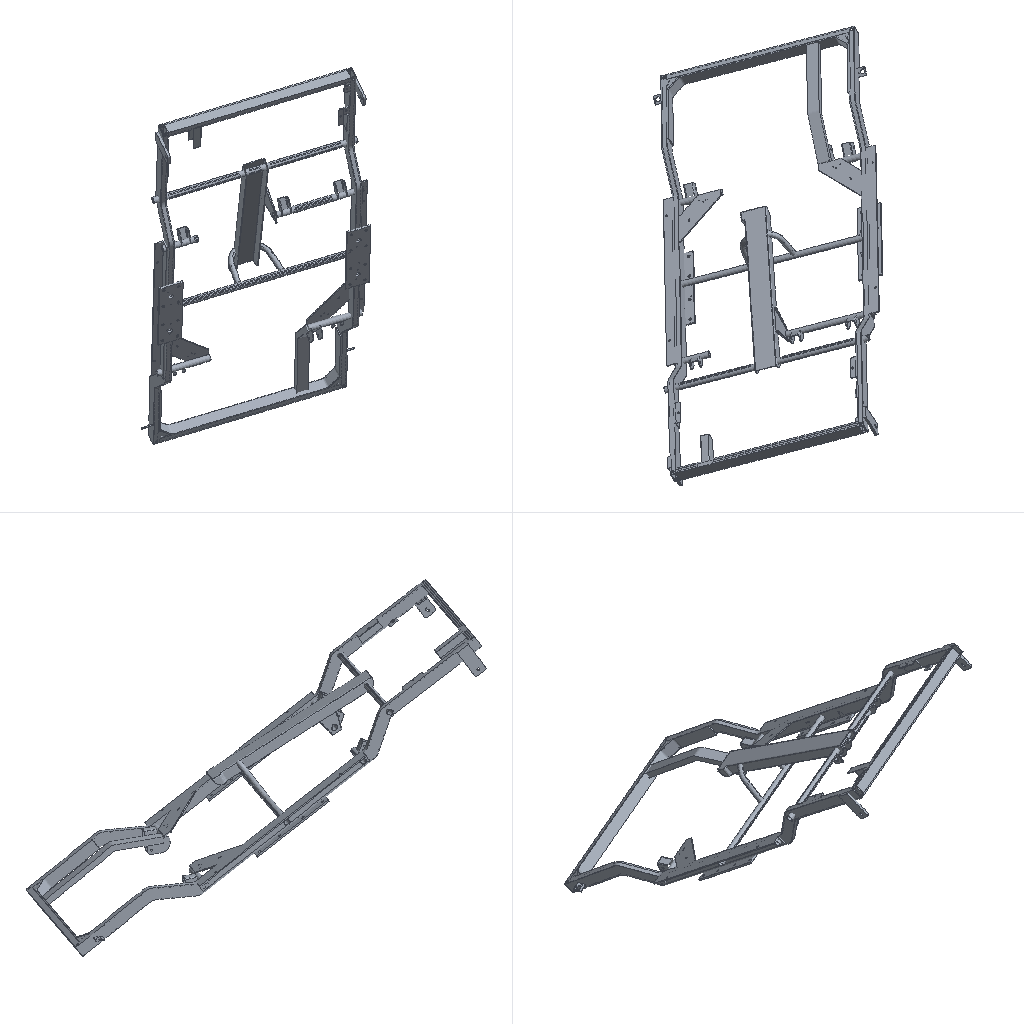Simulation study | ansys workbench
Set-up summary:
category,name,step,type,value,unit,region
solver,ansys_workbench
units,SI m-kg-s (Pa),,stated,"/units,MKS"
analysis,LS1,,static
load_step,LS1,LS1,static,nsubst=1; time=1
mesh,nodes,,,737056
mesh,elements,,,373772
element_type,SOLID187,,,242914
element_type,TARGE170,,,42796
element_type,CONTA174,,,42796
element_type,SOLID186,,,42166
element_type,SURF154,,,3100
material,Structural Steel,,E,2e+11,Pa
material,Structural Steel,,nu,0.3
material,Structural Steel,,density,7850,kg m^-3
material,Structural Steel,,conductivity,60.5,W m^-1 C^-1
material,Structural Steel,,specific_heat,434,J kg^-1 C^-1
material,Structural Steel,,cte,1.2e-05,C^-1
material,Structural Steel,,permeability,10000
material,Structural Steel,,resistivity,1.7e-07,kg m^3 A^-2 s^-3
load,Define Force Using Surface Effect Elements,LS1,surface-effect pres face 1,-51822.3,,SURF154 #195
load,Define Force Using Surface Effect Elements,LS1,surface-effect pres face 2,2.04463e+06,,SURF154 #195
load,Define Force Using Surface Effect Elements,LS1,surface-effect pres face 3,-1.57917e+06,,SURF154 #195
load,Define Force Using Surface Effect Elements,LS1,surface-effect pres face 1,-16714.4,,SURF154 #196
load,Define Force Using Surface Effect Elements,LS1,surface-effect pres face 2,1.2043e+06,,SURF154 #196
load,Define Force Using Surface Effect Elements,LS1,surface-effect pres face 3,-976255,,SURF154 #196
bc,Fixed Supports,model,fixed,[dofs=ALL],,_FIXEDSU
contact,Contact Region,,bonded (always),element=CONTA174
contact,Contact Region 2,,bonded (always),element=CONTA174
contact,Contact Region 3,,bonded (always),element=CONTA174
contact,Contact Region 4,,bonded (always),element=CONTA174
contact,Contact Region 5,,bonded (always),element=CONTA174
contact,Contact Region 6,,bonded (always),element=CONTA174
contact,Contact Region 7,,bonded (always),element=CONTA174
contact,Contact Region 8,,bonded (always),element=CONTA174
contact,Contact Region 9,,bonded (always),element=CONTA174
contact,Contact Region 10,,bonded (always),element=CONTA174
contact,Contact Region 11,,bonded (always),element=CONTA174
contact,Contact Region 12,,bonded (always),element=CONTA174
contact,Contact Region 13,,bonded (always),element=CONTA174
contact,Contact Region 14,,bonded (always),element=CONTA174
contact,Contact Region 15,,bonded (always),element=CONTA174
contact,Contact Region 16,,bonded (always),element=CONTA174
contact,Contact Region 17,,bonded (always),element=CONTA174
contact,Contact Region 18,,bonded (always),element=CONTA174
contact,Contact Region 19,,bonded (always),element=CONTA174
contact,Contact Region 20,,bonded (always),element=CONTA174
contact,Contact Region 21,,bonded (always),element=CONTA174
contact,Contact Region 22,,bonded (always),element=CONTA174
contact,Contact Region 23,,bonded (always),element=CONTA174
contact,Contact Region 24,,bonded (always),element=CONTA174
contact,Contact Region 25,,bonded (always),element=CONTA174
contact,Contact Region 26,,bonded (always),element=CONTA174
contact,Contact Region 27,,bonded (always),element=CONTA174
contact,Contact Region 28,,bonded (always),element=CONTA174
contact,Contact Region 29,,bonded (always),element=CONTA174
contact,Contact Region 30,,bonded (always),element=CONTA174
contact,Contact Region 31,,bonded (always),element=CONTA174
contact,Contact Region 32,,bonded (always),element=CONTA174
contact,Contact Region 33,,bonded (always),element=CONTA174
contact,Contact Region 34,,bonded (always),element=CONTA174
contact,Contact Region 35,,bonded (always),element=CONTA174
contact,Contact Region 36,,bonded (always),element=CONTA174
contact,Contact Region 37,,bonded (always),element=CONTA174
contact,Contact Region 38,,bonded (always),element=CONTA174
contact,Contact Region 39,,bonded (always),element=CONTA174
contact,Contact Region 40,,bonded (always),element=CONTA174
contact,Contact Region 41,,bonded (always),element=CONTA174
contact,Contact Region 42,,bonded (always),element=CONTA174
contact,Contact Region 43,,bonded (always),element=CONTA174
contact,Contact Region 44,,bonded (always),element=CONTA174
contact,Contact Region 45,,bonded (always),element=CONTA174
contact,Contact Region 46,,bonded (always),element=CONTA174
contact,Contact Region 47,,bonded (always),element=CONTA174
contact,Contact Region 48,,bonded (always),element=CONTA174
contact,Contact Region 49,,bonded (always),element=CONTA174
contact,Contact Region 50,,bonded (always),element=CONTA174
contact,Contact Region 51,,bonded (always),element=CONTA174
contact,Contact Region 52,,bonded (always),element=CONTA174
contact,Contact Region 53,,bonded (always),element=CONTA174
contact,Contact Region 54,,bonded (always),element=CONTA174
contact,Contact Region 55,,bonded (always),element=CONTA174
contact,Contact Region 56,,bonded (always),element=CONTA174
contact,Contact Region 57,,bonded (always),element=CONTA174
contact,Contact Region 58,,bonded (always),element=CONTA174
contact,Contact Region 59,,bonded (always),element=CONTA174
contact,Contact Region 60,,bonded (always),element=CONTA174
contact,Contact Region 61,,bonded (always),element=CONTA174
contact,Contact Region 62,,bonded (always),element=CONTA174
contact,Contact Region 63,,bonded (always),element=CONTA174
contact,Contact Region 64,,bonded (always),element=CONTA174
contact,Contact Region 65,,bonded (always),element=CONTA174
contact,Contact Region 66,,bonded (always),element=CONTA174
contact,Contact Region 67,,bonded (always),element=CONTA174
contact,Contact Region 68,,bonded (always),element=CONTA174
contact,Contact Region 69,,bonded (always),element=CONTA174
contact,Contact Region 70,,bonded (always),element=CONTA174
contact,Contact Region 71,,bonded (always),element=CONTA174
contact,Contact Region 72,,bonded (always),element=CONTA174
contact,Contact Region 73,,bonded (always),element=CONTA174
contact,Contact Region 74,,bonded (always),element=CONTA174
contact,Contact Region 75,,bonded (always),element=CONTA174
named_set,_FIXEDSU,,node,9496
Ansys APDL input file, long lists of numbers shortened:
/batch
/config,noeldb,1     ! force off writing results to database
*get,_wallstrt,active,,time,wall
! ANSYS input file written by Workbench version 2024 R2
! File used for geometry attach:
/title,wbnew--____ (A5)
! ****** Begin Custom Load Command Snippet ******
/COM, ACT Extensions:
/COM,     LSDYNA, 2024.2
/COM,/COM,     ANSYSMotion, 2024.2
/COM,
! ****** End   Custom Load Command Snippet ******
*DIM,_wb_ProjectScratch_dir,string,248
_wb_ProjectScratch_dir(1) = ''
*DIM,_wb_SolverFiles_dir,string,248
_wb_SolverFiles_dir(1) = ''
*DIM,_wb_userfiles_dir,string,248
_wb_userfiles_dir(1) = ''
/com,--- Data in consistent MKS units. See Solving Units in the help system for more information.
/units,MKS
/nopr
/wb,file,start              !  signify a WB generated input file
/prep7
! Turn off shape checking because checks already performed inside WB mesher.
! See help system for more information.
SHPP,OFF,,NOWARN
/nolist
etcon,set             ! allow ANSYS to choose best KEYOP's for 180x elements, resets any applicable keyopt to MAPDL defaults
/com,*********** Nodes for the whole assembly ***********
nblock,3,,810761
(1i9,3e20.9e3)
   685375    -3.735245650E-01     6.288331249E-01    -6.786277806E-01
! (737055 more lines like these left out)
-1
/wb,elem,start            !  set before creation of elements
/com,*********** Elements for Body 1 'car chassis-FreeParts|Shell1' ***********
et,1,186
keyo,1,2,1          ! set full integration on SOLID186
eblock,19,solid,,4650
(19i9)
        1        1        1        1        0        0        0        0       20        0        1     4393     4547     8424     8578     5014     5013     9044     9045
! (9299 more lines like these left out)
-1
/com,*********** Elements for Body 2 'car chassis-FreeParts|Body-Move/Copy6' ***********
et,2,187
eblock,19,solid,,1516
(19i9)
        2        2        2        2        0        0        0        0       10        0     4651    31992    32336    32302    32281    33664    34931    33663    33662
! (3031 more lines like these left out)
-1
/com,*********** Elements for Body 3 'car chassis-FreeParts|Extrude-Thin2' ***********
et,3,186
keyo,3,2,1          ! set full integration on SOLID186
eblock,19,solid,,3150
(19i9)
        3        3        3        3        0        0        0        0       20        0     6167    36484    36485    39633    39634    37878    37877    40677    40678
! (6299 more lines like these left out)
-1
/com,*********** Elements for Body 4 'car chassis-FreeParts|Cut-Extrude23' ***********
et,4,186
keyo,4,2,1          ! set full integration on SOLID186
eblock,19,solid,,106
(19i9)
        4        4        4        4        0        0        0        0       20        0     9317    55081    55102    55101    55100    55140    55119    55120    55121
! (211 more lines like these left out)
-1
/com,*********** Elements for Body 5 'car chassis-FreeParts|Mirror1[5]' ***********
et,5,186
keyo,5,2,1          ! set full integration on SOLID186
eblock,19,solid,,1800
(19i9)
        5        5        5        5        0        0        0        0       20        0     9423    55832    55833    55835    55840    57226    57225    57223    57218
! (3599 more lines like these left out)
-1
/com,*********** Elements for Body 6 'car chassis-FreeParts|Sweep-Thin1' ***********
et,6,187
eblock,19,solid,,3008
(19i9)
        6        6        6        6        0        0        0        0       10        0    11223    64352    64602    64609    64752    65503    67232    65504    65506
! (6015 more lines like these left out)
-1
/com,*********** Elements for Body 7 'car chassis-FreeParts|Mirror1[1]' ***********
et,7,187
eblock,19,solid,,1712
(19i9)
        7        7        7        7        0        0        0        0       10        0    14231    70826    71059    71007    71076    73222    73989    73221    73223
! (3423 more lines like these left out)
-1
/com,*********** Elements for Body 8 'car chassis-FreeParts|Boss-Extrude21' ***********
et,8,186
keyo,8,2,1          ! set full integration on SOLID186
eblock,19,solid,,24
(19i9)
        8        8        8        8        0        0        0        0       20        0    15943    74065    74073    74093    74097    74069    74072    74092    74094
! (47 more lines like these left out)
-1
/com,*********** Elements for Body 9 'car chassis-FreeParts|Body-Move/Copy5' ***********
et,9,187
eblock,19,solid,,1521
(19i9)
        9        9        9        9        0        0        0        0       10        0    15967    74233    74605    74549    74532    74851    76559    74848    74847
! (3041 more lines like these left out)
-1
/com,*********** Elements for Body 10 'car chassis-FreeParts|Fillet12' ***********
et,10,187
eblock,19,solid,,421
(19i9)
       10       10       10       10        0        0        0        0       10        0    17488    77605    77645    77616    77672    78178    78224    78174    78179
! (841 more lines like these left out)
-1
/com,*********** Elements for Body 11 'car chassis-FreeParts|Cut-Extrude16' ***********
et,11,187
eblock,19,solid,,1518
(19i9)
       11       11       11       11        0        0        0        0       10        0    17909    78484    78485    78647    78620    79603    79617    79608    79605
! (3035 more lines like these left out)
-1
/com,*********** Elements for Body 12 'car chassis-FreeParts|Cut-Extrude2' ***********
et,12,186
keyo,12,2,1         ! set full integration on SOLID186
eblock,19,solid,,124
(19i9)
       12       12       12       12        0        0        0        0       20        0    19427    81667    81668    81704    81674    81742    81741    81705    81735
! (247 more lines like these left out)
-1
/com,*********** Elements for Body 13 'car chassis-FreeParts|Extrude-Thin4' ***********
et,13,186
keyo,13,2,1         ! set full integration on SOLID186
eblock,19,solid,,3132
(19i9)
       13       13       13       13        0        0        0        0       20        0    19551    83574    87054    87053    83575    83581    87059    87060    83582
! (6263 more lines like these left out)
-1
/com,*********** Elements for Body 14 'car chassis-FreeParts|Mirror1[4]' ***********
et,14,186
keyo,14,2,1         ! set full integration on SOLID186
eblock,19,solid,,773
(19i9)
       14       14       14       14        0        0        0        0       20        0    22683   102990   103020   103132   103133   103277   103247   103135   103134
! (1545 more lines like these left out)
-1
/com,*********** Elements for Body 15 'car chassis-FreeParts|Mirror3' ***********
et,15,187
eblock,19,solid,,3010
(19i9)
       15       15       15       15        0        0        0        0       10        0    23456   108364   108576   108388   108377   110721   110967   110712   110711
! (6019 more lines like these left out)
-1
/com,*********** Elements for Body 16 'car chassis-FreeParts|Mirror1[7]' ***********
et,16,186
keyo,16,2,1         ! set full integration on SOLID186
eblock,19,solid,,80
(19i9)
       16       16       16       16        0        0        0        0       20        0    26466   114286   114335   114334   114398   114302   114327   114328   114396
! (159 more lines like these left out)
-1
/com,*********** Elements for Body 17 'car chassis-FreeParts|Boss-Extrude16' ***********
et,17,186
keyo,17,2,1         ! set full integration on SOLID186
eblock,19,solid,,624
(19i9)
       17       17       17       17        0        0        0        0       20        0    26546   115451   115485   115511   115637   115460   115486   115512   115638
! (1247 more lines like these left out)
-1
/com,*********** Elements for Body 18 'car chassis-FreeParts|Cut-Extrude5' ***********
et,18,187
eblock,19,solid,,1527
(19i9)
       18       18       18       18        0        0        0        0       10        0    27170   119503   119538   119968   119776   120806   120976   120809   120808
! (3053 more lines like these left out)
-1
/com,*********** Elements for Body 19 'car chassis-FreeParts|Shell3' ***********
et,19,187
eblock,19,solid,,71914
(19i9)
       19       19       19       19        0        0        0        0       10        0    28697   122954   146330   122979   122965   148277   148438   148274   148273
! (143827 more lines like these left out)
-1
/com,*********** Elements for Body 20 'car chassis-FreeParts|Boss-Extrude4' ***********
et,20,186
keyo,20,2,1         ! set full integration on SOLID186
eblock,19,solid,,5600
(19i9)
       20       20       20       20        0        0        0        0       20        0   100611   264773   271074   271062   271012   269212   271110   271061   271021
! (11199 more lines like these left out)
-1
/com,*********** Elements for Body 21 'car chassis-FreeParts|Cut-Extrude19' ***********
et,21,187
eblock,19,solid,,32876
(19i9)
       21       21       21       21        0        0        0        0       10        0   106211   292671   293638   292975   303848   304198   306550   304196   304201
! (65751 more lines like these left out)
-1
/com,*********** Elements for Body 22 'car chassis-FreeParts|Extrude-Thin12' ***********
et,22,186
keyo,22,2,1         ! set full integration on SOLID186
eblock,19,solid,,5380
(19i9)
       22       22       22       22        0        0        0        0       20        0   139087   359310   365520   365518   365453   361989   365529   365519   365509
! (10759 more lines like these left out)
-1
/com,*********** Elements for Body 23 'car chassis-FreeParts|Extrude-Thin9' ***********
et,23,186
keyo,23,2,1         ! set full integration on SOLID186
eblock,19,solid,,540
(19i9)
       23       23       23       23        0        0        0        0       20        0   144467   391412   391413   391951   391952   391646   391645   392125   392126
! (1079 more lines like these left out)
-1
/com,*********** Elements for Body 24 'car chassis-FreeParts|Cut-Extrude13[1]' ***********
et,24,187
eblock,19,solid,,20919
(19i9)
       24       24       24       24        0        0        0        0       10        0   145007   395852   401161   396791   397764   409238   415890   409232   409236
! (41837 more lines like these left out)
-1
/com,*********** Elements for Body 25 'car chassis-FreeParts|Boss-Extrude10' ***********
et,25,186
keyo,25,2,1         ! set full integration on SOLID186
eblock,19,solid,,1665
(19i9)
       25       25       25       25        0        0        0        0       20        0   165926   434165   434166   434172   434190   435469   435468   435462   435444
! (3329 more lines like these left out)
-1
/com,*********** Elements for Body 26 'car chassis-FreeParts|Extrude-Thin3' ***********
et,26,186
keyo,26,2,1         ! set full integration on SOLID186
eblock,19,solid,,1368
(19i9)
       26       26       26       26        0        0        0        0       20        0   167591   442738   444256   444255   442739   442745   444263   444264   442746
! (2735 more lines like these left out)
-1
/com,*********** Elements for Body 27 'car chassis-FreeParts|Cut-Extrude21[2]' ***********
et,27,186
keyo,27,2,1         ! set full integration on SOLID186
eblock,19,solid,,3000
(19i9)
       27       27       27       27        0        0        0        0       20        0   168959   451283   452270   452269   452283   453428   452441   452442   452428
! (5999 more lines like these left out)
-1
/com,*********** Elements for Body 28 'car chassis-FreeParts|Mirror4' ***********
et,28,187
eblock,19,solid,,1614
(19i9)
       28       28       28       28        0        0        0        0       10        0   171959   468557   469153   468559   468897   469274   469284   469268   469273
! (3227 more lines like these left out)
-1
! (1 more sections like these left out)
/com,*********** Elements for Body 30 'car chassis-FreeParts|Boss-Extrude15' ***********
et,30,186
keyo,30,2,1         ! set full integration on SOLID186
eblock,19,solid,,590
(19i9)
       30       30       30       30        0        0        0        0       20        0   173665   472683   472716   472802   472803   473148   473115   473029   473028
! (1179 more lines like these left out)
-1
/com,*********** Elements for Body 31 'car chassis-FreeParts|Body-Move/Copy7' ***********
et,31,187
eblock,19,solid,,409
(19i9)
       31       31       31       31        0        0        0        0       10        0   174255   476289   476385   476293   476360   476691   476714   476688   476690
! (817 more lines like these left out)
-1
! (3 more sections like these left out)
/com,*********** Elements for Body 35 'car chassis-FreeParts|Mirror1[8]' ***********
et,35,186
keyo,35,2,1         ! set full integration on SOLID186
eblock,19,solid,,124
(19i9)
       35       35       35       35        0        0        0        0       20        0   178094   489044   489269   489053   489047   489119   489282   489110   489116
! (247 more lines like these left out)
-1
/com,*********** Elements for Body 36 'car chassis-FreeParts|Shell4' ***********
et,36,187
eblock,19,solid,,71996
(19i9)
       36       36       36       36        0        0        0        0       10        0   178218   490599   511935   512117   513547   518014   629890   518015   518016
! (143991 more lines like these left out)
-1
! (1 more sections like these left out)
/com,*********** Elements for Body 38 'car chassis-FreeParts|Shell2' ***********
et,38,186
keyo,38,2,1         ! set full integration on SOLID186
eblock,19,solid,,4650
(19i9)
       38       38       38       38        0        0        0        0       20        0   250294   634481   634635   639440   639594   635098   635099   639596   639595
! (9299 more lines like these left out)
-1
! (4 more sections like these left out)
/com,*********** Elements for Body 43 'car chassis-FreeParts|Mirror2' ***********
et,43,186
keyo,43,2,1         ! set full integration on SOLID186
eblock,19,solid,,598
(19i9)
       43       43       43       43        0        0        0        0       20        0   263584   694153   694256   694320   694254   694666   694563   694499   694565
! (1195 more lines like these left out)
-1
/com,*********** Elements for Body 44 'car chassis-FreeParts|Cut-Extrude13[3]' ***********
et,44,187
eblock,19,solid,,20899
(19i9)
       44       44       44       44        0        0        0        0       10        0   264182   699092   704235   699644   704188   713468   717616   713461   713467
! (41797 more lines like these left out)
-1
/wb,elem,end               !  done creating elements
/com,*********** Send User Defined Coordinate System(s) ***********
csys,0
toffst,273.15,      ! Temperature offset from absolute zero
/com,*********** Set Reference Temperature ***********
tref,22.
/wb,mat,start              !  starting to send materials
/com,*********** Send Materials ***********
Temperature = 'TEMP' ! Temperature
MP,DENS,1,7850,	! kg m^-3
MP,ALPX,1,1.2e-05,	! C^-1
MP,C,1,434,	! J kg^-1 C^-1
MP,KXX,1,60.5,	! W m^-1 C^-1
MP,RSVX,1,1.7e-07,	! kg m^3 A^-2 s^-3
MP,EX,1,200000000000,	! Pa
MP,NUXY,1,0.3,
MP,MURX,1,10000,
Temperature = 'TEMP' ! Temperature
MP,DENS,2,7850,	! kg m^-3
MP,ALPX,2,1.2e-05,	! C^-1
MP,C,2,434,	! J kg^-1 C^-1
MP,KXX,2,60.5,	! W m^-1 C^-1
MP,RSVX,2,1.7e-07,	! kg m^3 A^-2 s^-3
MP,EX,2,200000000000,	! Pa
MP,NUXY,2,0.3,
MP,MURX,2,10000,
Temperature = 'TEMP' ! Temperature
MP,DENS,3,7850,	! kg m^-3
MP,ALPX,3,1.2e-05,	! C^-1
MP,C,3,434,	! J kg^-1 C^-1
MP,KXX,3,60.5,	! W m^-1 C^-1
MP,RSVX,3,1.7e-07,	! kg m^3 A^-2 s^-3
MP,EX,3,200000000000,	! Pa
MP,NUXY,3,0.3,
MP,MURX,3,10000,
Temperature = 'TEMP' ! Temperature
MP,DENS,4,7850,	! kg m^-3
MP,ALPX,4,1.2e-05,	! C^-1
MP,C,4,434,	! J kg^-1 C^-1
MP,KXX,4,60.5,	! W m^-1 C^-1
MP,RSVX,4,1.7e-07,	! kg m^3 A^-2 s^-3
MP,EX,4,200000000000,	! Pa
MP,NUXY,4,0.3,
MP,MURX,4,10000,
Temperature = 'TEMP' ! Temperature
MP,DENS,5,7850,	! kg m^-3
MP,ALPX,5,1.2e-05,	! C^-1
MP,C,5,434,	! J kg^-1 C^-1
MP,KXX,5,60.5,	! W m^-1 C^-1
MP,RSVX,5,1.7e-07,	! kg m^3 A^-2 s^-3
MP,EX,5,200000000000,	! Pa
MP,NUXY,5,0.3,
MP,MURX,5,10000,
Temperature = 'TEMP' ! Temperature
MP,DENS,6,7850,	! kg m^-3
MP,ALPX,6,1.2e-05,	! C^-1
MP,C,6,434,	! J kg^-1 C^-1
MP,KXX,6,60.5,	! W m^-1 C^-1
MP,RSVX,6,1.7e-07,	! kg m^3 A^-2 s^-3
MP,EX,6,200000000000,	! Pa
MP,NUXY,6,0.3,
MP,MURX,6,10000,
Temperature = 'TEMP' ! Temperature
MP,DENS,7,7850,	! kg m^-3
MP,ALPX,7,1.2e-05,	! C^-1
MP,C,7,434,	! J kg^-1 C^-1
MP,KXX,7,60.5,	! W m^-1 C^-1
MP,RSVX,7,1.7e-07,	! kg m^3 A^-2 s^-3
MP,EX,7,200000000000,	! Pa
MP,NUXY,7,0.3,
MP,MURX,7,10000,
Temperature = 'TEMP' ! Temperature
MP,DENS,8,7850,	! kg m^-3
MP,ALPX,8,1.2e-05,	! C^-1
MP,C,8,434,	! J kg^-1 C^-1
MP,KXX,8,60.5,	! W m^-1 C^-1
MP,RSVX,8,1.7e-07,	! kg m^3 A^-2 s^-3
MP,EX,8,200000000000,	! Pa
MP,NUXY,8,0.3,
MP,MURX,8,10000,
Temperature = 'TEMP' ! Temperature
MP,DENS,9,7850,	! kg m^-3
MP,ALPX,9,1.2e-05,	! C^-1
MP,C,9,434,	! J kg^-1 C^-1
MP,KXX,9,60.5,	! W m^-1 C^-1
MP,RSVX,9,1.7e-07,	! kg m^3 A^-2 s^-3
MP,EX,9,200000000000,	! Pa
! (317 more lines like these left out)
/wb,mat,end                !  done sending materials
!************************* Model Summary ********************
!car chassis-FreeParts|Shell1,	ç»æé¢,	matid,	1
!car chassis-FreeParts|Body-Move/Copy6,	ç»æé¢,	matid,	2
!car chassis-FreeParts|Extrude-Thin2,	ç»æé¢,	matid,	3
! (43 more lines like these left out)
*get,_xmin,node,,mnloc,x
*get,_ymin,node,,mnloc,y
*get,_zmin,node,,mnloc,z
*get,_xmax,node,,mxloc,x
*get,_ymax,node,,mxloc,y
*get,_zmax,node,,mxloc,z
_ASMDIAG=(_xmax-_xmin)*(_xmax-_xmin)+(_ymax-_ymin)*(_ymax-_ymin)+(_zmax-_zmin)*(_zmax-_zmin)
_ASMDIAG=SQRT(_ASMDIAG)
/wb,contact,start          !  starting to send contact
/com,*********** Create Contact "½Ó´¥ÇøÓò" ***********
/com,            Real Constant Set For Above Contact Is 46 & 45
*set,tid,46
*set,cid,45
r,tid
r,cid
et,tid,170
et,cid,174
eblock,10,,,81
(15i9)
   498067       46       46       46        0     4071     4072     3918     3917    20898    20440    20436    20437
! (80 more lines like these left out)
-1
eblock,10,,,81
(15i9)
   498148       45       45       45        0     4071     4072     3918     3917    20898    20440    20436    20437
! (80 more lines like these left out)
-1
eblock,10,,,22
(15i9)
   498229       45       46       45        0    81843    81833    81855    81856    82384    82385    82422    82407
! (21 more lines like these left out)
-1
eblock,10,,,22
(15i9)
   498251       46       45       46        0    81843    81833    81855    81856    82384    82385    82422    82407
! (21 more lines like these left out)
-1
keyo,cid,8,2               ! auto create asymmetric contact (from Program Controlled setting)
keyo,cid,10,0              ! adjust contact stiffness each NR iteration (from Program Controlled setting)
keyo,cid,12,5              ! bonded always
keyo,cid,18,1              ! small sliding turned on by application
keyo,cid,2,2               ! MPC for bonded contacts (from Program Controlled setting)
keyo,tid,5,0               ! Automatic constraint type detection
keyo,cid,4,2               ! on nodal point - normal to target surface (from Program Controlled setting)
keyo,cid,9,1               ! ignore initial gaps/penetration
keyo,cid,7,0               ! No Prediction
rmod,tid,3,10.      ! FKN
rmod,tid,5,0.       ! ICONT
rmod,tid,6,0.       ! PINB
rmod,tid,10,0.      ! CNOF
rmod,tid,12,0.      ! FKT
rmod,tid,36,155     ! WB DSID
rmod,cid,3,10.      ! FKN
rmod,cid,5,0.       ! ICONT
rmod,cid,6,0.       ! PINB
rmod,cid,10,0.      ! CNOF
rmod,cid,12,0.      ! FKT
rmod,cid,36,155     ! WB DSID
/com,*********** Create Contact "½Ó´¥ÇøÓò 2" ***********
/com,            Real Constant Set For Above Contact Is 48 & 47
*set,tid,48
*set,cid,47
r,tid
r,cid
et,tid,170
et,cid,174
eblock,10,,,78
(15i9)
   498273       48       48       48        0       27     3624     1919       45     9133    14764     9170     9132
! (77 more lines like these left out)
-1
eblock,10,,,78
(15i9)
   498351       47       47       47        0       27     3624     1919       45     9133    14764     9170     9132
! (77 more lines like these left out)
-1
eblock,10,,,80
(15i9)
   498429       47       48       47        0   114344   114351   114260   114261   114675   114418   114416   114421
! (79 more lines like these left out)
-1
eblock,10,,,80
(15i9)
   498509       48       47       48        0   114344   114351   114260   114261   114675   114418   114416   114421
! (79 more lines like these left out)
-1
keyo,cid,8,2               ! auto create asymmetric contact (from Program Controlled setting)
keyo,cid,10,0              ! adjust contact stiffness each NR iteration (from Program Controlled setting)
keyo,cid,12,5              ! bonded always
keyo,cid,18,1              ! small sliding turned on by application
keyo,cid,2,2               ! MPC for bonded contacts (from Program Controlled setting)
keyo,tid,5,0               ! Automatic constraint type detection
keyo,cid,4,2               ! on nodal point - normal to target surface (from Program Controlled setting)
keyo,cid,9,1               ! ignore initial gaps/penetration
keyo,cid,7,0               ! No Prediction
rmod,tid,3,10.      ! FKN
rmod,tid,5,0.       ! ICONT
rmod,tid,6,0.       ! PINB
rmod,tid,10,0.      ! CNOF
rmod,tid,12,0.      ! FKT
rmod,tid,36,158     ! WB DSID
rmod,cid,3,10.      ! FKN
rmod,cid,5,0.       ! ICONT
rmod,cid,6,0.       ! PINB
rmod,cid,10,0.      ! CNOF
rmod,cid,12,0.      ! FKT
rmod,cid,36,158     ! WB DSID
/com,*********** Create Contact "½Ó´¥ÇøÓò 3" ***********
/com,            Real Constant Set For Above Contact Is 50 & 49
*set,tid,50
*set,cid,49
r,tid
r,cid
et,tid,170
et,cid,174
eblock,10,,,30
(15i9)
   498589       50       50       50        0     9043     9044     5013     5013    31762    23723     5013    23722
! (29 more lines like these left out)
-1
eblock,10,,,30
(15i9)
   498619       49       49       49        0     9043     9044     5013     5013    31762    23723     5013    23722
! (29 more lines like these left out)
-1
eblock,10,,,205
(15i9)
   498649       49       50       49        0   133272   134310   133704   133704   223948   225982   133704   223947
! (204 more lines like these left out)
-1
eblock,10,,,205
(15i9)
   498854       50       49       50        0   133272   134310   133704   133704   223948   225982   133704   223947
! (204 more lines like these left out)
-1
keyo,cid,8,2               ! auto create asymmetric contact (from Program Controlled setting)
keyo,cid,10,0              ! adjust contact stiffness each NR iteration (from Program Controlled setting)
keyo,cid,12,5              ! bonded always
keyo,cid,18,1              ! small sliding turned on by application
keyo,cid,2,2               ! MPC for bonded contacts (from Program Controlled setting)
keyo,tid,5,0               ! Automatic constraint type detection
keyo,cid,4,2               ! on nodal point - normal to target surface (from Program Controlled setting)
keyo,cid,9,1               ! ignore initial gaps/penetration
keyo,cid,7,0               ! No Prediction
rmod,tid,3,10.      ! FKN
rmod,tid,5,0.       ! ICONT
rmod,tid,6,0.       ! PINB
rmod,tid,10,0.      ! CNOF
rmod,tid,12,0.      ! FKT
rmod,tid,36,161     ! WB DSID
rmod,cid,3,10.      ! FKN
rmod,cid,5,0.       ! ICONT
rmod,cid,6,0.       ! PINB
rmod,cid,10,0.      ! CNOF
rmod,cid,12,0.      ! FKT
rmod,cid,36,161     ! WB DSID
/com,*********** Create Contact "½Ó´¥ÇøÓò 4" ***********
/com,            Real Constant Set For Above Contact Is 52 & 51
*set,tid,52
*set,cid,51
r,tid
r,cid
et,tid,170
et,cid,174
eblock,10,,,176
(15i9)
   499059       52       52       52        0     4353     4354     4200     4199    21744    21286    21282    21283
! (175 more lines like these left out)
-1
eblock,10,,,176
(15i9)
   499235       51       51       51        0     4353     4354     4200     4199    21744    21286    21282    21283
! (175 more lines like these left out)
-1
eblock,10,,,50
(15i9)
   499411       51       52       51        0   269889   269891   269950   269890   288170   288174   288171   288169
! (49 more lines like these left out)
-1
eblock,10,,,50
(15i9)
   499461       52       51       52        0   269889   269891   269950   269890   288170   288174   288171   288169
! (49 more lines like these left out)
-1
keyo,cid,8,2               ! auto create asymmetric contact (from Program Controlled setting)
keyo,cid,10,0              ! adjust contact stiffness each NR iteration (from Program Controlled setting)
keyo,cid,12,5              ! bonded always
keyo,cid,18,1              ! small sliding turned on by application
keyo,cid,2,2               ! MPC for bonded contacts (from Program Controlled setting)
keyo,tid,5,0               ! Automatic constraint type detection
keyo,cid,4,2               ! on nodal point - normal to target surface (from Program Controlled setting)
keyo,cid,9,1               ! ignore initial gaps/penetration
keyo,cid,7,0               ! No Prediction
rmod,tid,3,10.      ! FKN
rmod,tid,5,0.       ! ICONT
rmod,tid,6,0.       ! PINB
rmod,tid,10,0.      ! CNOF
rmod,tid,12,0.      ! FKT
rmod,tid,36,164     ! WB DSID
rmod,cid,3,10.      ! FKN
rmod,cid,5,0.       ! ICONT
rmod,cid,6,0.       ! PINB
rmod,cid,10,0.      ! CNOF
rmod,cid,12,0.      ! FKT
rmod,cid,36,164     ! WB DSID
/com,*********** Create Contact "½Ó´¥ÇøÓò 5" ***********
/com,            Real Constant Set For Above Contact Is 54 & 53
*set,tid,54
*set,cid,53
r,tid
r,cid
et,tid,170
et,cid,174
eblock,10,,,1448
(15i9)
   499511       54       54       54        0     3782     3783     3629     3628    20031    19573    19569    19570
! (1447 more lines like these left out)
-1
eblock,10,,,1448
(15i9)
   500959       53       53       53        0     3782     3783     3629     3628    20031    19573    19569    19570
! (1447 more lines like these left out)
-1
eblock,10,,,1390
(15i9)
   502407       53       54       53        0   363511   363520   362597   362728   382201   380436   380435   380697
! (1389 more lines like these left out)
-1
eblock,10,,,1390
(15i9)
   503797       54       53       54        0   363511   363520   362597   362728   382201   380436   380435   380697
! (1389 more lines like these left out)
-1
keyo,cid,8,2               ! auto create asymmetric contact (from Program Controlled setting)
keyo,cid,10,0              ! adjust contact stiffness each NR iteration (from Program Controlled setting)
keyo,cid,12,5              ! bonded always
keyo,cid,18,1              ! small sliding turned on by application
keyo,cid,2,2               ! MPC for bonded contacts (from Program Controlled setting)
keyo,tid,5,0               ! Automatic constraint type detection
keyo,cid,4,2               ! on nodal point - normal to target surface (from Program Controlled setting)
keyo,cid,9,1               ! ignore initial gaps/penetration
keyo,cid,7,0               ! No Prediction
rmod,tid,3,10.      ! FKN
rmod,tid,5,0.       ! ICONT
rmod,tid,6,0.       ! PINB
rmod,tid,10,0.      ! CNOF
rmod,tid,12,0.      ! FKT
rmod,tid,36,167     ! WB DSID
rmod,cid,3,10.      ! FKN
rmod,cid,5,0.       ! ICONT
rmod,cid,6,0.       ! PINB
rmod,cid,10,0.      ! CNOF
rmod,cid,12,0.      ! FKT
rmod,cid,36,167     ! WB DSID
! (70 more sections like these left out)
/wb,contact,end            !  done creating contacts
/golist
/wb,load,start             !  starting to send loads
/com,*********** Fixed Supports ***********
CMBLOCK,_FIXEDSU,NODE,     9496
(8i10)
    452356    452357    452358    452359    452360    452361    452362    452363
! (1186 more lines like these left out)
cmsel,s,_FIXEDSU
d,all,all
nsel,all
/com,*********** Define Force Using Surface Effect Elements ***********
local,12,0,0.,0.,0.,0.,0.,0.
csys,0
et,195,154
mat,195
eblock,10,,,1550
(15i9)
   583659      195      195      195       12   632599   636188   635257   632606   641713   649645   641727   641712
! (1549 more lines like these left out)
-1
esel,s,type,,195
keyop,195,2,1       ! Apply load in local coordinate system
keyop,195,7,1       ! Use original area so load is constant in large deformation
esel,all
/com,*********** Define Force Using Surface Effect Elements ***********
local,13,0,0.,0.,0.,0.,0.,0.
csys,0
et,196,154
mat,196
eblock,10,,,1550
(15i9)
   585209      196      196      196       13       44     2229      989       58     9168    11980     9194     9167
! (1549 more lines like these left out)
-1
esel,s,type,,196
keyop,196,2,1       ! Apply load in local coordinate system
keyop,196,7,1       ! Use original area so load is constant in large deformation
esel,all
/gst,on,on
fini
*get,_numnode,node,0,count
*get,_numelem,elem,0,count
*get, _MAXELEMNUM, elem, 0, NUM, MAX
*get, _MAXNODENUM, node, 0, NUM, MAX
*get, _MAXELEMTYPE, etyp, 0, NUM, MAX
*get, _MAXREALCONST, rcon, 0, NUM, MAX
/go
/wb,load,end               !  done creating loads
/com,--- Number of total nodes = %_numnode%
/com,--- Number of contact elements = 88692
/com,--- Number of spring elements = 0
/com,--- Number of bearing elements = 0
/com,--- Number of solid elements = 285080
/com,--- Number of condensed parts = 0
/com,--- Number of total elements = %_numelem%
*get,_wallbsol,active,,time,wall
/com,****************************************************************************
/com,*************************    SOLUTION       ********************************
/com,****************************************************************************
/solu
antype,0                   ! static analysis
_thickRatio=0.0682  ! Ratio of thick parts in the model
eqsl,sparse,,,,,1
cntr,print,1               ! print out contact info and also make no initial contact an error
dmpoption,emat,no             ! Don't combine emat file for DANSYS
dmpoption,esav,no             ! Don't combine esav file for DANSYS
nldiag,cont,iter           ! print out contact info each equilibrium iteration
rescontrol,,none                 ! Do not keep any restart files
/com,****************************************************
/com,******************* SOLVE FOR LS 1 OF 1 ****************
esel,s,type,,195
nsle
sfe,all,1,pres,1,-51822.292
sfe,all,2,pres,1,2044625.369
sfe,all,3,pres,1,-1579167.769
esel,s,type,,196
nsle
sfe,all,1,pres,1,-16714.443
sfe,all,2,pres,1,1204304.547
sfe,all,3,pres,1,-976254.589
nsel,all
esel,all
/nopr
/gopr
nsub,1,1,1
time,1.
outres,erase
outres,all,none
outres,nsol,all,
outres,rsol,all
outres,eangl,all
outres,etmp,all
outres,veng,all
outres,strs,all,
outres,epel,all,
outres,eppl,all,
outres,cont,all,
! *********** WB SOLVE COMMAND ***********
! check interactive state
*get,ANSINTER_,active,,int
*if,ANSINTER_,ne,0,then
/eof
*endif
solve
/com *************** Write FE CONNECTORS *********
CEWRITE,file,ce,,INTE
/com,****************************************************
/com,*************** FINISHED SOLVE FOR LS 1 *************
*get,_wallasol,active,,time,wall
/nopr
*get,_numnode,node,0,count
*get,_numelem,elem,0,count
*get, _MAXELEMNUM, elem, 0, NUM, MAX
*get, _MAXNODENUM, node, 0, NUM, MAX,,,INTERNAL
*get, _MAXELEMTYPE, etyp, 0, NUM, MAX
*get, _MAXREALCONST, rcon, 0, NUM, MAX
*get,_NSOLTHREADS,active,0,ntfs
*get,_NSOLPROCESSES,active,0,npfs
/gopr
/post1
xmlo,ENCODING,ISO-8859-1
xmlo,parm
/xml,parm,xml
fini
/gopr
*get,_walldone,active,,time,wall
_preptime=(_wallbsol-_wallstrt)*3600
_solvtime=(_wallasol-_wallbsol)*3600
_posttime=(_walldone-_wallasol)*3600
_totaltim=(_walldone-_wallstrt)*3600
*get,_dlbratio,active,0,solu,dlbr
*get,_combtime,active,0,solu,comb
*get,_ssmode,active,0,solu,ssmm
*get,_ndofs,active,0,solu,ndof
*get,_sol_end_time,active,0,set,time
*if,_sol_end_time,eq,1.,then
/fclean				!clean distributed files
*endif
/com,--- Total number of nodes = %_numnode%
/com,--- Total number of elements = %_numelem%
/com,--- Element load balance ratio = %_dlbratio%
/com,--- Time to combine distributed files = %_combtime%
/com,--- Sparse memory mode = %_ssmode%
/com,--- Number of DOF = %_ndofs%
/wb,file,end               ! done with WB generated input
Results summary:
result,analyses[0].index,,,1
result,analyses[0].system,,,SYS
result,analyses[0].deck,,,deck.dat
result,analyses[0].solve_status,,,completed
result,analyses[0].analysis_type,,,static
result,analyses[0].physics,,,mechanical
result,analyses[0].unit_system,,,"MKS: m, kg, N, s, V, A, degC"
result,analyses[0].n_sets,,,1
result,analyses[0].load_steps[0].set,set=1,,1
result,analyses[0].load_steps[0].time_or_freq,set=1,,1
result,analyses[0].load_steps[0].max_displacement_magnitude,set=1,,0.04909
result,analyses[0].load_steps[0].max_von_mises_nodal,set=1,,9.08394e+09
result,analyses[0].load_steps[0].reaction_force_sum_xyz[1],set=1,,2652.37
result,analyses[0].load_steps[0].reaction_force_sum_xyz[2],set=1,,-125734
result,analyses[0].load_steps[0].reaction_force_sum_xyz[3],set=1,,98894.8